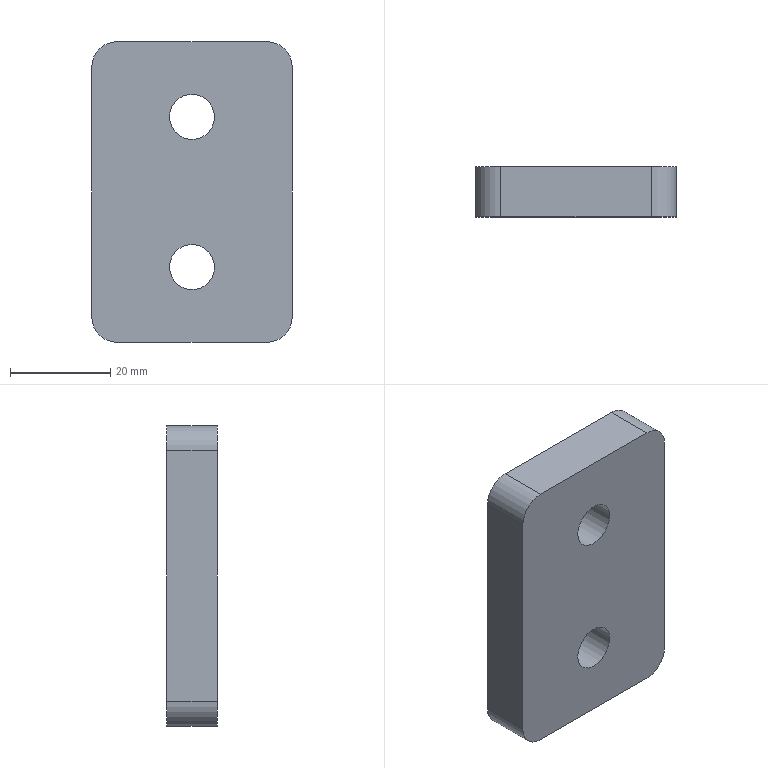Part | STEP file | SN10_002_011_PLACA | 1 solid | 12 faces | box 40 x 10 x 60 mm | volume 22513 mm3 | cylinder 6 | plane 6 | commonest cylinder face diameters 10 x4 9 x2
STEP:
#1=CARTESIAN_POINT('',(0.,0.,0.));
#2=DIRECTION('',(0.,0.,1.));
#3=DIRECTION('',(1.,0.,0.));
#4=AXIS2_PLACEMENT_3D('',#1,#2,#3);
#5=CARTESIAN_POINT('',(893.949,30.,-122.843));
#6=VERTEX_POINT('',#5);
#7=CARTESIAN_POINT('',(890.,30.,-125.));
#8=DIRECTION('',(0.,1.,0.));
#9=DIRECTION('',(1.,0.,0.));
#10=AXIS2_PLACEMENT_3D('',#7,#8,#9);
#11=CIRCLE('',#10,4.5);
#12=CARTESIAN_POINT('',(890.,29.9,-125.));
#13=DIRECTION('',(0.,-1.,0.));
#14=DIRECTION('',(0.8776,0.,0.4794));
#15=AXIS2_PLACEMENT_3D('',#12,#13,#14);
#16=CYLINDRICAL_SURFACE('',#15,4.5);
#17=CARTESIAN_POINT('',(12.066,-0.1));
#18=DIRECTION('',(-1.,0.));
#19=VECTOR('',#18,1.);
#20=LINE('',#17,#19);
#21=(GEOMETRIC_REPRESENTATION_CONTEXT(2)PARAMETRIC_REPRESENTATION_CONTEXT()REPRESENTATION_CONTEXT('',''));
#22=DEFINITIONAL_REPRESENTATION('',(#20),#21);
#23=PCURVE('',#16,#22);
#24=CARTESIAN_POINT('',(0.,30.,0.));
#25=DIRECTION('',(0.,1.,0.));
#26=DIRECTION('',(0.,0.,1.));
#27=AXIS2_PLACEMENT_3D('',#24,#25,#26);
#28=PLANE('',#27);
#29=CARTESIAN_POINT('',(-125.,890.));
#30=DIRECTION('',(0.,1.));
#31=AXIS2_PLACEMENT_2D('',#29,#30);
#32=CIRCLE('',#31,4.5);
#33=(GEOMETRIC_REPRESENTATION_CONTEXT(2)PARAMETRIC_REPRESENTATION_CONTEXT()REPRESENTATION_CONTEXT('',''));
#34=DEFINITIONAL_REPRESENTATION('',(#32),#33);
#35=PCURVE('',#28,#34);
#36=SURFACE_CURVE('',#11,(#23,#35),.PCURVE_S1.);
#37=EDGE_CURVE('',#6,#6,#36,.T.);
#38=ORIENTED_EDGE('',*,*,#37,.F.);
#39=CARTESIAN_POINT('',(893.949,20.,-122.843));
#40=VERTEX_POINT('',#39);
#41=CARTESIAN_POINT('',(893.949,30.,-122.843));
#42=CARTESIAN_POINT('',(893.949,20.,-122.843));
#43=B_SPLINE_CURVE_WITH_KNOTS('',1,(#41,#42),.UNSPECIFIED.,.F.,.F.,(2,2),(-0.1,9.9),.PIECEWISE_BEZIER_KNOTS.);
#44=CARTESIAN_POINT('',(6.283,0.));
#45=DIRECTION('',(0.,1.));
#46=VECTOR('',#45,1.);
#47=LINE('',#44,#46);
#48=(GEOMETRIC_REPRESENTATION_CONTEXT(2)PARAMETRIC_REPRESENTATION_CONTEXT()REPRESENTATION_CONTEXT('',''));
#49=DEFINITIONAL_REPRESENTATION('',(#47),#48);
#50=PCURVE('',#16,#49);
#51=CARTESIAN_POINT('',(0.,0.));
#52=DIRECTION('',(0.,1.));
#53=VECTOR('',#52,1.);
#54=LINE('',#51,#53);
#55=(GEOMETRIC_REPRESENTATION_CONTEXT(2)PARAMETRIC_REPRESENTATION_CONTEXT()REPRESENTATION_CONTEXT('',''));
#56=DEFINITIONAL_REPRESENTATION('',(#54),#55);
#57=PCURVE('',#16,#56);
#58=SEAM_CURVE('',#43,(#50,#57),.PCURVE_S1.);
#59=EDGE_CURVE('',#6,#40,#58,.T.);
#60=ORIENTED_EDGE('',*,*,#59,.T.);
#61=CARTESIAN_POINT('',(890.,20.,-125.));
#62=DIRECTION('',(0.,-1.,0.));
#63=DIRECTION('',(1.,0.,0.));
#64=AXIS2_PLACEMENT_3D('',#61,#62,#63);
#65=CIRCLE('',#64,4.5);
#66=CARTESIAN_POINT('',(-0.5,9.9));
#67=DIRECTION('',(1.,0.));
#68=VECTOR('',#67,1.);
#69=LINE('',#66,#68);
#70=(GEOMETRIC_REPRESENTATION_CONTEXT(2)PARAMETRIC_REPRESENTATION_CONTEXT()REPRESENTATION_CONTEXT('',''));
#71=DEFINITIONAL_REPRESENTATION('',(#69),#70);
#72=PCURVE('',#16,#71);
#73=CARTESIAN_POINT('',(0.,20.,0.));
#74=DIRECTION('',(0.,1.,0.));
#75=DIRECTION('',(0.,0.,1.));
#76=AXIS2_PLACEMENT_3D('',#73,#74,#75);
#77=PLANE('',#76);
#78=CARTESIAN_POINT('',(-125.,894.5));
#79=CARTESIAN_POINT('',(-117.206,894.5));
#80=CARTESIAN_POINT('',(-121.103,887.75));
#81=CARTESIAN_POINT('',(-125.,881.));
#82=CARTESIAN_POINT('',(-128.897,887.75));
#83=CARTESIAN_POINT('',(-132.794,894.5));
#84=CARTESIAN_POINT('',(-125.,894.5));
#85=(BOUNDED_CURVE()B_SPLINE_CURVE(2,(#78,#79,#80,#81,#82,#83,#84),.UNSPECIFIED.,.T.,.F.)B_SPLINE_CURVE_WITH_KNOTS((1,2,2,2,2,1),(-2.094,0.,2.094,4.189,6.283,8.378),.UNSPECIFIED.)CURVE()GEOMETRIC_REPRESENTATION_ITEM()RATIONAL_B_SPLINE_CURVE((1.,0.5,1.,0.5,1.,0.5,1.))REPRESENTATION_ITEM(''));
#86=(GEOMETRIC_REPRESENTATION_CONTEXT(2)PARAMETRIC_REPRESENTATION_CONTEXT()REPRESENTATION_CONTEXT('',''));
#87=DEFINITIONAL_REPRESENTATION('',(#85),#86);
#88=PCURVE('',#77,#87);
#89=SURFACE_CURVE('',#65,(#72,#88),.PCURVE_S1.);
#90=EDGE_CURVE('',#40,#40,#89,.T.);
#91=ORIENTED_EDGE('',*,*,#90,.F.);
#92=ORIENTED_EDGE('',*,*,#59,.F.);
#93=EDGE_LOOP('',(#38,#60,#91,#92));
#94=FACE_BOUND('',#93,.F.);
#95=ADVANCED_FACE('',(#94),#16,.F.);
#96=CARTESIAN_POINT('',(875.,30.,-140.));
#97=VERTEX_POINT('',#96);
#98=CARTESIAN_POINT('',(905.,30.,-140.));
#99=VERTEX_POINT('',#98);
#100=CARTESIAN_POINT('',(875.,30.,-140.));
#101=DIRECTION('',(1.,0.,0.));
#102=VECTOR('',#101,1.);
#103=LINE('',#100,#102);
#104=CARTESIAN_POINT('',(-140.,875.));
#105=DIRECTION('',(0.,1.));
#106=VECTOR('',#105,1.);
#107=LINE('',#104,#106);
#108=(GEOMETRIC_REPRESENTATION_CONTEXT(2)PARAMETRIC_REPRESENTATION_CONTEXT()REPRESENTATION_CONTEXT('',''));
#109=DEFINITIONAL_REPRESENTATION('',(#107),#108);
#110=PCURVE('',#28,#109);
#111=CARTESIAN_POINT('',(870.,20.,-140.));
#112=DIRECTION('',(0.,0.,1.));
#113=DIRECTION('',(1.,0.,0.));
#114=AXIS2_PLACEMENT_3D('',#111,#112,#113);
#115=PLANE('',#114);
#116=CARTESIAN_POINT('',(5.,10.));
#117=DIRECTION('',(1.,0.));
#118=VECTOR('',#117,1.);
#119=LINE('',#116,#118);
#120=(GEOMETRIC_REPRESENTATION_CONTEXT(2)PARAMETRIC_REPRESENTATION_CONTEXT()REPRESENTATION_CONTEXT('',''));
#121=DEFINITIONAL_REPRESENTATION('',(#119),#120);
#122=PCURVE('',#115,#121);
#123=SURFACE_CURVE('',#103,(#110,#122),.PCURVE_S1.);
#124=EDGE_CURVE('',#97,#99,#123,.T.);
#125=ORIENTED_EDGE('',*,*,#124,.F.);
#126=CARTESIAN_POINT('',(870.,30.,-135.));
#127=VERTEX_POINT('',#126);
#128=CARTESIAN_POINT('',(875.,30.,-135.));
#129=DIRECTION('',(0.,1.,0.));
#130=DIRECTION('',(1.,0.,0.));
#131=AXIS2_PLACEMENT_3D('',#128,#129,#130);
#132=CIRCLE('',#131,5.);
#133=CARTESIAN_POINT('',(-135.,875.));
#134=DIRECTION('',(0.,1.));
#135=AXIS2_PLACEMENT_2D('',#133,#134);
#136=CIRCLE('',#135,5.);
#137=(GEOMETRIC_REPRESENTATION_CONTEXT(2)PARAMETRIC_REPRESENTATION_CONTEXT()REPRESENTATION_CONTEXT('',''));
#138=DEFINITIONAL_REPRESENTATION('',(#136),#137);
#139=PCURVE('',#28,#138);
#140=CARTESIAN_POINT('',(875.,25.,-135.));
#141=DIRECTION('',(0.,1.,0.));
#142=DIRECTION('',(0.,0.,-1.));
#143=AXIS2_PLACEMENT_3D('',#140,#141,#142);
#144=CYLINDRICAL_SURFACE('',#143,5.);
#145=CARTESIAN_POINT('',(-1.571,5.));
#146=DIRECTION('',(1.,0.));
#147=VECTOR('',#146,1.);
#148=LINE('',#145,#147);
#149=(GEOMETRIC_REPRESENTATION_CONTEXT(2)PARAMETRIC_REPRESENTATION_CONTEXT()REPRESENTATION_CONTEXT('',''));
#150=DEFINITIONAL_REPRESENTATION('',(#148),#149);
#151=PCURVE('',#144,#150);
#152=SURFACE_CURVE('',#132,(#139,#151),.PCURVE_S1.);
#153=EDGE_CURVE('',#97,#127,#152,.T.);
#154=ORIENTED_EDGE('',*,*,#153,.T.);
#155=CARTESIAN_POINT('',(870.,30.,-85.));
#156=VERTEX_POINT('',#155);
#157=CARTESIAN_POINT('',(870.,30.,-85.));
#158=DIRECTION('',(0.,0.,-1.));
#159=VECTOR('',#158,1.);
#160=LINE('',#157,#159);
#161=CARTESIAN_POINT('',(-85.,870.));
#162=DIRECTION('',(-1.,0.));
#163=VECTOR('',#162,1.);
#164=LINE('',#161,#163);
#165=(GEOMETRIC_REPRESENTATION_CONTEXT(2)PARAMETRIC_REPRESENTATION_CONTEXT()REPRESENTATION_CONTEXT('',''));
#166=DEFINITIONAL_REPRESENTATION('',(#164),#165);
#167=PCURVE('',#28,#166);
#168=CARTESIAN_POINT('',(870.,20.,-80.));
#169=DIRECTION('',(1.,0.,0.));
#170=DIRECTION('',(0.,0.,-1.));
#171=AXIS2_PLACEMENT_3D('',#168,#169,#170);
#172=PLANE('',#171);
#173=CARTESIAN_POINT('',(5.,10.));
#174=DIRECTION('',(1.,0.));
#175=VECTOR('',#174,1.);
#176=LINE('',#173,#175);
#177=(GEOMETRIC_REPRESENTATION_CONTEXT(2)PARAMETRIC_REPRESENTATION_CONTEXT()REPRESENTATION_CONTEXT('',''));
#178=DEFINITIONAL_REPRESENTATION('',(#176),#177);
#179=PCURVE('',#172,#178);
#180=SURFACE_CURVE('',#160,(#167,#179),.PCURVE_S1.);
#181=EDGE_CURVE('',#156,#127,#180,.T.);
#182=ORIENTED_EDGE('',*,*,#181,.F.);
#183=CARTESIAN_POINT('',(875.,30.,-80.));
#184=VERTEX_POINT('',#183);
#185=CARTESIAN_POINT('',(875.,30.,-85.));
#186=DIRECTION('',(0.,1.,0.));
#187=DIRECTION('',(1.,0.,0.));
#188=AXIS2_PLACEMENT_3D('',#185,#186,#187);
#189=CIRCLE('',#188,5.);
#190=CARTESIAN_POINT('',(-85.,875.));
#191=DIRECTION('',(0.,1.));
#192=AXIS2_PLACEMENT_2D('',#190,#191);
#193=CIRCLE('',#192,5.);
#194=(GEOMETRIC_REPRESENTATION_CONTEXT(2)PARAMETRIC_REPRESENTATION_CONTEXT()REPRESENTATION_CONTEXT('',''));
#195=DEFINITIONAL_REPRESENTATION('',(#193),#194);
#196=PCURVE('',#28,#195);
#197=CARTESIAN_POINT('',(875.,25.,-85.));
#198=DIRECTION('',(0.,1.,0.));
#199=DIRECTION('',(-1.,0.,0.));
#200=AXIS2_PLACEMENT_3D('',#197,#198,#199);
#201=CYLINDRICAL_SURFACE('',#200,5.);
#202=CARTESIAN_POINT('',(-3.142,5.));
#203=DIRECTION('',(1.,0.));
#204=VECTOR('',#203,1.);
#205=LINE('',#202,#204);
#206=(GEOMETRIC_REPRESENTATION_CONTEXT(2)PARAMETRIC_REPRESENTATION_CONTEXT()REPRESENTATION_CONTEXT('',''));
#207=DEFINITIONAL_REPRESENTATION('',(#205),#206);
#208=PCURVE('',#201,#207);
#209=SURFACE_CURVE('',#189,(#196,#208),.PCURVE_S1.);
#210=EDGE_CURVE('',#156,#184,#209,.T.);
#211=ORIENTED_EDGE('',*,*,#210,.T.);
#212=CARTESIAN_POINT('',(905.,30.,-80.));
#213=VERTEX_POINT('',#212);
#214=CARTESIAN_POINT('',(905.,30.,-80.));
#215=DIRECTION('',(-1.,0.,0.));
#216=VECTOR('',#215,1.);
#217=LINE('',#214,#216);
#218=CARTESIAN_POINT('',(-80.,905.));
#219=DIRECTION('',(0.,-1.));
#220=VECTOR('',#219,1.);
#221=LINE('',#218,#220);
#222=(GEOMETRIC_REPRESENTATION_CONTEXT(2)PARAMETRIC_REPRESENTATION_CONTEXT()REPRESENTATION_CONTEXT('',''));
#223=DEFINITIONAL_REPRESENTATION('',(#221),#222);
#224=PCURVE('',#28,#223);
#225=CARTESIAN_POINT('',(910.,20.,-80.));
#226=DIRECTION('',(0.,0.,-1.));
#227=DIRECTION('',(-1.,0.,0.));
#228=AXIS2_PLACEMENT_3D('',#225,#226,#227);
#229=PLANE('',#228);
#230=CARTESIAN_POINT('',(5.,10.));
#231=DIRECTION('',(1.,0.));
#232=VECTOR('',#231,1.);
#233=LINE('',#230,#232);
#234=(GEOMETRIC_REPRESENTATION_CONTEXT(2)PARAMETRIC_REPRESENTATION_CONTEXT()REPRESENTATION_CONTEXT('',''));
#235=DEFINITIONAL_REPRESENTATION('',(#233),#234);
#236=PCURVE('',#229,#235);
#237=SURFACE_CURVE('',#217,(#224,#236),.PCURVE_S1.);
#238=EDGE_CURVE('',#213,#184,#237,.T.);
#239=ORIENTED_EDGE('',*,*,#238,.F.);
#240=CARTESIAN_POINT('',(910.,30.,-85.));
#241=VERTEX_POINT('',#240);
#242=CARTESIAN_POINT('',(905.,30.,-85.));
#243=DIRECTION('',(0.,1.,0.));
#244=DIRECTION('',(1.,0.,0.));
#245=AXIS2_PLACEMENT_3D('',#242,#243,#244);
#246=CIRCLE('',#245,5.);
#247=CARTESIAN_POINT('',(-85.,905.));
#248=DIRECTION('',(0.,1.));
#249=AXIS2_PLACEMENT_2D('',#247,#248);
#250=CIRCLE('',#249,5.);
#251=(GEOMETRIC_REPRESENTATION_CONTEXT(2)PARAMETRIC_REPRESENTATION_CONTEXT()REPRESENTATION_CONTEXT('',''));
#252=DEFINITIONAL_REPRESENTATION('',(#250),#251);
#253=PCURVE('',#28,#252);
#254=CARTESIAN_POINT('',(905.,25.,-85.));
#255=DIRECTION('',(0.,1.,0.));
#256=DIRECTION('',(0.,0.,1.));
#257=AXIS2_PLACEMENT_3D('',#254,#255,#256);
#258=CYLINDRICAL_SURFACE('',#257,5.);
#259=CARTESIAN_POINT('',(-4.712,5.));
#260=DIRECTION('',(1.,0.));
#261=VECTOR('',#260,1.);
#262=LINE('',#259,#261);
#263=(GEOMETRIC_REPRESENTATION_CONTEXT(2)PARAMETRIC_REPRESENTATION_CONTEXT()REPRESENTATION_CONTEXT('',''));
#264=DEFINITIONAL_REPRESENTATION('',(#262),#263);
#265=PCURVE('',#258,#264);
#266=SURFACE_CURVE('',#246,(#253,#265),.PCURVE_S1.);
#267=EDGE_CURVE('',#213,#241,#266,.T.);
#268=ORIENTED_EDGE('',*,*,#267,.T.);
#269=CARTESIAN_POINT('',(910.,30.,-135.));
#270=VERTEX_POINT('',#269);
#271=CARTESIAN_POINT('',(910.,30.,-135.));
#272=DIRECTION('',(0.,0.,1.));
#273=VECTOR('',#272,1.);
#274=LINE('',#271,#273);
#275=CARTESIAN_POINT('',(-135.,910.));
#276=DIRECTION('',(1.,0.));
#277=VECTOR('',#276,1.);
#278=LINE('',#275,#277);
#279=(GEOMETRIC_REPRESENTATION_CONTEXT(2)PARAMETRIC_REPRESENTATION_CONTEXT()REPRESENTATION_CONTEXT('',''));
#280=DEFINITIONAL_REPRESENTATION('',(#278),#279);
#281=PCURVE('',#28,#280);
#282=CARTESIAN_POINT('',(910.,20.,-140.));
#283=DIRECTION('',(-1.,0.,0.));
#284=DIRECTION('',(0.,0.,1.));
#285=AXIS2_PLACEMENT_3D('',#282,#283,#284);
#286=PLANE('',#285);
#287=CARTESIAN_POINT('',(5.,10.));
#288=DIRECTION('',(1.,0.));
#289=VECTOR('',#288,1.);
#290=LINE('',#287,#289);
#291=(GEOMETRIC_REPRESENTATION_CONTEXT(2)PARAMETRIC_REPRESENTATION_CONTEXT()REPRESENTATION_CONTEXT('',''));
#292=DEFINITIONAL_REPRESENTATION('',(#290),#291);
#293=PCURVE('',#286,#292);
#294=SURFACE_CURVE('',#274,(#281,#293),.PCURVE_S1.);
#295=EDGE_CURVE('',#270,#241,#294,.T.);
#296=ORIENTED_EDGE('',*,*,#295,.F.);
#297=CARTESIAN_POINT('',(905.,30.,-135.));
#298=DIRECTION('',(0.,1.,0.));
#299=DIRECTION('',(1.,0.,0.));
#300=AXIS2_PLACEMENT_3D('',#297,#298,#299);
#301=CIRCLE('',#300,5.);
#302=CARTESIAN_POINT('',(-135.,905.));
#303=DIRECTION('',(0.,1.));
#304=AXIS2_PLACEMENT_2D('',#302,#303);
#305=CIRCLE('',#304,5.);
#306=(GEOMETRIC_REPRESENTATION_CONTEXT(2)PARAMETRIC_REPRESENTATION_CONTEXT()REPRESENTATION_CONTEXT('',''));
#307=DEFINITIONAL_REPRESENTATION('',(#305),#306);
#308=PCURVE('',#28,#307);
#309=CARTESIAN_POINT('',(905.,25.,-135.));
#310=DIRECTION('',(0.,1.,0.));
#311=DIRECTION('',(1.,0.,0.));
#312=AXIS2_PLACEMENT_3D('',#309,#310,#311);
#313=CYLINDRICAL_SURFACE('',#312,5.);
#314=CARTESIAN_POINT('',(0.,5.));
#315=DIRECTION('',(1.,0.));
#316=VECTOR('',#315,1.);
#317=LINE('',#314,#316);
#318=(GEOMETRIC_REPRESENTATION_CONTEXT(2)PARAMETRIC_REPRESENTATION_CONTEXT()REPRESENTATION_CONTEXT('',''));
#319=DEFINITIONAL_REPRESENTATION('',(#317),#318);
#320=PCURVE('',#313,#319);
#321=SURFACE_CURVE('',#301,(#308,#320),.PCURVE_S1.);
#322=EDGE_CURVE('',#270,#99,#321,.T.);
#323=ORIENTED_EDGE('',*,*,#322,.T.);
#324=EDGE_LOOP('',(#125,#154,#182,#211,#239,#268,#296,#323));
#325=FACE_BOUND('',#324,.T.);
#326=ORIENTED_EDGE('',*,*,#37,.F.);
#327=EDGE_LOOP('',(#326));
#328=FACE_BOUND('',#327,.T.);
#329=CARTESIAN_POINT('',(893.949,30.,-92.843));
#330=VERTEX_POINT('',#329);
#331=CARTESIAN_POINT('',(890.,30.,-95.));
#332=DIRECTION('',(0.,1.,0.));
#333=DIRECTION('',(1.,0.,0.));
#334=AXIS2_PLACEMENT_3D('',#331,#332,#333);
#335=CIRCLE('',#334,4.5);
#336=CARTESIAN_POINT('',(-95.,890.));
#337=DIRECTION('',(0.,1.));
#338=AXIS2_PLACEMENT_2D('',#336,#337);
#339=CIRCLE('',#338,4.5);
#340=(GEOMETRIC_REPRESENTATION_CONTEXT(2)PARAMETRIC_REPRESENTATION_CONTEXT()REPRESENTATION_CONTEXT('',''));
#341=DEFINITIONAL_REPRESENTATION('',(#339),#340);
#342=PCURVE('',#28,#341);
#343=CARTESIAN_POINT('',(890.,29.9,-95.));
#344=DIRECTION('',(0.,-1.,0.));
#345=DIRECTION('',(0.8776,0.,0.4794));
#346=AXIS2_PLACEMENT_3D('',#343,#344,#345);
#347=CYLINDRICAL_SURFACE('',#346,4.5);
#348=CARTESIAN_POINT('',(12.066,-0.1));
#349=DIRECTION('',(-1.,0.));
#350=VECTOR('',#349,1.);
#351=LINE('',#348,#350);
#352=(GEOMETRIC_REPRESENTATION_CONTEXT(2)PARAMETRIC_REPRESENTATION_CONTEXT()REPRESENTATION_CONTEXT('',''));
#353=DEFINITIONAL_REPRESENTATION('',(#351),#352);
#354=PCURVE('',#347,#353);
#355=SURFACE_CURVE('',#335,(#342,#354),.PCURVE_S1.);
#356=EDGE_CURVE('',#330,#330,#355,.T.);
#357=ORIENTED_EDGE('',*,*,#356,.F.);
#358=EDGE_LOOP('',(#357));
#359=FACE_BOUND('',#358,.T.);
#360=ADVANCED_FACE('',(#325,#328,#359),#28,.T.);
#361=CARTESIAN_POINT('',(905.,20.,-140.));
#362=VERTEX_POINT('',#361);
#363=CARTESIAN_POINT('',(905.,20.,-140.));
#364=DIRECTION('',(0.,1.,0.));
#365=VECTOR('',#364,1.);
#366=LINE('',#363,#365);
#367=CARTESIAN_POINT('',(35.,0.));
#368=DIRECTION('',(0.,1.));
#369=VECTOR('',#368,1.);
#370=LINE('',#367,#369);
#371=(GEOMETRIC_REPRESENTATION_CONTEXT(2)PARAMETRIC_REPRESENTATION_CONTEXT()REPRESENTATION_CONTEXT('',''));
#372=DEFINITIONAL_REPRESENTATION('',(#370),#371);
#373=PCURVE('',#115,#372);
#374=CARTESIAN_POINT('',(1.571,-5.));
#375=DIRECTION('',(0.,1.));
#376=VECTOR('',#375,1.);
#377=LINE('',#374,#376);
#378=(GEOMETRIC_REPRESENTATION_CONTEXT(2)PARAMETRIC_REPRESENTATION_CONTEXT()REPRESENTATION_CONTEXT('',''));
#379=DEFINITIONAL_REPRESENTATION('',(#377),#378);
#380=PCURVE('',#313,#379);
#381=SURFACE_CURVE('',#366,(#373,#380),.PCURVE_S1.);
#382=EDGE_CURVE('',#362,#99,#381,.T.);
#383=ORIENTED_EDGE('',*,*,#382,.F.);
#384=CARTESIAN_POINT('',(875.,20.,-140.));
#385=VERTEX_POINT('',#384);
#386=CARTESIAN_POINT('',(875.,20.,-140.));
#387=DIRECTION('',(1.,0.,0.));
#388=VECTOR('',#387,1.);
#389=LINE('',#386,#388);
#390=CARTESIAN_POINT('',(5.,0.));
#391=DIRECTION('',(1.,0.));
#392=VECTOR('',#391,1.);
#393=LINE('',#390,#392);
#394=(GEOMETRIC_REPRESENTATION_CONTEXT(2)PARAMETRIC_REPRESENTATION_CONTEXT()REPRESENTATION_CONTEXT('',''));
#395=DEFINITIONAL_REPRESENTATION('',(#393),#394);
#396=PCURVE('',#115,#395);
#397=CARTESIAN_POINT('',(-140.,875.));
#398=DIRECTION('',(0.,1.));
#399=VECTOR('',#398,1.);
#400=LINE('',#397,#399);
#401=(GEOMETRIC_REPRESENTATION_CONTEXT(2)PARAMETRIC_REPRESENTATION_CONTEXT()REPRESENTATION_CONTEXT('',''));
#402=DEFINITIONAL_REPRESENTATION('',(#400),#401);
#403=PCURVE('',#77,#402);
#404=SURFACE_CURVE('',#389,(#396,#403),.PCURVE_S1.);
#405=EDGE_CURVE('',#385,#362,#404,.T.);
#406=ORIENTED_EDGE('',*,*,#405,.F.);
#407=CARTESIAN_POINT('',(875.,20.,-140.));
#408=DIRECTION('',(0.,1.,0.));
#409=VECTOR('',#408,1.);
#410=LINE('',#407,#409);
#411=CARTESIAN_POINT('',(5.,0.));
#412=DIRECTION('',(0.,1.));
#413=VECTOR('',#412,1.);
#414=LINE('',#411,#413);
#415=(GEOMETRIC_REPRESENTATION_CONTEXT(2)PARAMETRIC_REPRESENTATION_CONTEXT()REPRESENTATION_CONTEXT('',''));
#416=DEFINITIONAL_REPRESENTATION('',(#414),#415);
#417=PCURVE('',#115,#416);
#418=CARTESIAN_POINT('',(0.,-5.));
#419=DIRECTION('',(0.,1.));
#420=VECTOR('',#419,1.);
#421=LINE('',#418,#420);
#422=(GEOMETRIC_REPRESENTATION_CONTEXT(2)PARAMETRIC_REPRESENTATION_CONTEXT()REPRESENTATION_CONTEXT('',''));
#423=DEFINITIONAL_REPRESENTATION('',(#421),#422);
#424=PCURVE('',#144,#423);
#425=SURFACE_CURVE('',#410,(#417,#424),.PCURVE_S1.);
#426=EDGE_CURVE('',#385,#97,#425,.T.);
#427=ORIENTED_EDGE('',*,*,#426,.T.);
#428=ORIENTED_EDGE('',*,*,#124,.T.);
#429=EDGE_LOOP('',(#383,#406,#427,#428));
#430=FACE_BOUND('',#429,.T.);
#431=ADVANCED_FACE('',(#430),#115,.F.);
#432=CARTESIAN_POINT('',(870.,20.,-135.));
#433=VERTEX_POINT('',#432);
#434=CARTESIAN_POINT('',(870.,20.,-135.));
#435=DIRECTION('',(0.,1.,0.));
#436=VECTOR('',#435,1.);
#437=LINE('',#434,#436);
#438=CARTESIAN_POINT('',(55.,0.));
#439=DIRECTION('',(0.,1.));
#440=VECTOR('',#439,1.);
#441=LINE('',#438,#440);
#442=(GEOMETRIC_REPRESENTATION_CONTEXT(2)PARAMETRIC_REPRESENTATION_CONTEXT()REPRESENTATION_CONTEXT('',''));
#443=DEFINITIONAL_REPRESENTATION('',(#441),#442);
#444=PCURVE('',#172,#443);
#445=CARTESIAN_POINT('',(1.571,-5.));
#446=DIRECTION('',(0.,1.));
#447=VECTOR('',#446,1.);
#448=LINE('',#445,#447);
#449=(GEOMETRIC_REPRESENTATION_CONTEXT(2)PARAMETRIC_REPRESENTATION_CONTEXT()REPRESENTATION_CONTEXT('',''));
#450=DEFINITIONAL_REPRESENTATION('',(#448),#449);
#451=PCURVE('',#144,#450);
#452=SURFACE_CURVE('',#437,(#444,#451),.PCURVE_S1.);
#453=EDGE_CURVE('',#433,#127,#452,.T.);
#454=ORIENTED_EDGE('',*,*,#453,.F.);
#455=CARTESIAN_POINT('',(870.,20.,-85.));
#456=VERTEX_POINT('',#455);
#457=CARTESIAN_POINT('',(870.,20.,-85.));
#458=DIRECTION('',(0.,0.,-1.));
#459=VECTOR('',#458,1.);
#460=LINE('',#457,#459);
#461=CARTESIAN_POINT('',(5.,0.));
#462=DIRECTION('',(1.,0.));
#463=VECTOR('',#462,1.);
#464=LINE('',#461,#463);
#465=(GEOMETRIC_REPRESENTATION_CONTEXT(2)PARAMETRIC_REPRESENTATION_CONTEXT()REPRESENTATION_CONTEXT('',''));
#466=DEFINITIONAL_REPRESENTATION('',(#464),#465);
#467=PCURVE('',#172,#466);
#468=CARTESIAN_POINT('',(-85.,870.));
#469=DIRECTION('',(-1.,0.));
#470=VECTOR('',#469,1.);
#471=LINE('',#468,#470);
#472=(GEOMETRIC_REPRESENTATION_CONTEXT(2)PARAMETRIC_REPRESENTATION_CONTEXT()REPRESENTATION_CONTEXT('',''));
#473=DEFINITIONAL_REPRESENTATION('',(#471),#472);
#474=PCURVE('',#77,#473);
#475=SURFACE_CURVE('',#460,(#467,#474),.PCURVE_S1.);
#476=EDGE_CURVE('',#456,#433,#475,.T.);
#477=ORIENTED_EDGE('',*,*,#476,.F.);
#478=CARTESIAN_POINT('',(870.,20.,-85.));
#479=DIRECTION('',(0.,1.,0.));
#480=VECTOR('',#479,1.);
#481=LINE('',#478,#480);
#482=CARTESIAN_POINT('',(5.,0.));
#483=DIRECTION('',(0.,1.));
#484=VECTOR('',#483,1.);
#485=LINE('',#482,#484);
#486=(GEOMETRIC_REPRESENTATION_CONTEXT(2)PARAMETRIC_REPRESENTATION_CONTEXT()REPRESENTATION_CONTEXT('',''));
#487=DEFINITIONAL_REPRESENTATION('',(#485),#486);
#488=PCURVE('',#172,#487);
#489=CARTESIAN_POINT('',(0.,-5.));
#490=DIRECTION('',(0.,1.));
#491=VECTOR('',#490,1.);
#492=LINE('',#489,#491);
#493=(GEOMETRIC_REPRESENTATION_CONTEXT(2)PARAMETRIC_REPRESENTATION_CONTEXT()REPRESENTATION_CONTEXT('',''));
#494=DEFINITIONAL_REPRESENTATION('',(#492),#493);
#495=PCURVE('',#201,#494);
#496=SURFACE_CURVE('',#481,(#488,#495),.PCURVE_S1.);
#497=EDGE_CURVE('',#456,#156,#496,.T.);
#498=ORIENTED_EDGE('',*,*,#497,.T.);
#499=ORIENTED_EDGE('',*,*,#181,.T.);
#500=EDGE_LOOP('',(#454,#477,#498,#499));
#501=FACE_BOUND('',#500,.T.);
#502=ADVANCED_FACE('',(#501),#172,.F.);
#503=CARTESIAN_POINT('',(875.,20.,-80.));
#504=VERTEX_POINT('',#503);
#505=CARTESIAN_POINT('',(875.,20.,-80.));
#506=DIRECTION('',(0.,1.,0.));
#507=VECTOR('',#506,1.);
#508=LINE('',#505,#507);
#509=CARTESIAN_POINT('',(35.,0.));
#510=DIRECTION('',(0.,1.));
#511=VECTOR('',#510,1.);
#512=LINE('',#509,#511);
#513=(GEOMETRIC_REPRESENTATION_CONTEXT(2)PARAMETRIC_REPRESENTATION_CONTEXT()REPRESENTATION_CONTEXT('',''));
#514=DEFINITIONAL_REPRESENTATION('',(#512),#513);
#515=PCURVE('',#229,#514);
#516=CARTESIAN_POINT('',(1.571,-5.));
#517=DIRECTION('',(0.,1.));
#518=VECTOR('',#517,1.);
#519=LINE('',#516,#518);
#520=(GEOMETRIC_REPRESENTATION_CONTEXT(2)PARAMETRIC_REPRESENTATION_CONTEXT()REPRESENTATION_CONTEXT('',''));
#521=DEFINITIONAL_REPRESENTATION('',(#519),#520);
#522=PCURVE('',#201,#521);
#523=SURFACE_CURVE('',#508,(#515,#522),.PCURVE_S1.);
#524=EDGE_CURVE('',#504,#184,#523,.T.);
#525=ORIENTED_EDGE('',*,*,#524,.F.);
#526=CARTESIAN_POINT('',(905.,20.,-80.));
#527=VERTEX_POINT('',#526);
#528=CARTESIAN_POINT('',(905.,20.,-80.));
#529=DIRECTION('',(-1.,0.,0.));
#530=VECTOR('',#529,1.);
#531=LINE('',#528,#530);
#532=CARTESIAN_POINT('',(5.,0.));
#533=DIRECTION('',(1.,0.));
#534=VECTOR('',#533,1.);
#535=LINE('',#532,#534);
#536=(GEOMETRIC_REPRESENTATION_CONTEXT(2)PARAMETRIC_REPRESENTATION_CONTEXT()REPRESENTATION_CONTEXT('',''));
#537=DEFINITIONAL_REPRESENTATION('',(#535),#536);
#538=PCURVE('',#229,#537);
#539=CARTESIAN_POINT('',(-80.,905.));
#540=DIRECTION('',(0.,-1.));
#541=VECTOR('',#540,1.);
#542=LINE('',#539,#541);
#543=(GEOMETRIC_REPRESENTATION_CONTEXT(2)PARAMETRIC_REPRESENTATION_CONTEXT()REPRESENTATION_CONTEXT('',''));
#544=DEFINITIONAL_REPRESENTATION('',(#542),#543);
#545=PCURVE('',#77,#544);
#546=SURFACE_CURVE('',#531,(#538,#545),.PCURVE_S1.);
#547=EDGE_CURVE('',#527,#504,#546,.T.);
#548=ORIENTED_EDGE('',*,*,#547,.F.);
#549=CARTESIAN_POINT('',(905.,20.,-80.));
#550=DIRECTION('',(0.,1.,0.));
#551=VECTOR('',#550,1.);
#552=LINE('',#549,#551);
#553=CARTESIAN_POINT('',(5.,0.));
#554=DIRECTION('',(0.,1.));
#555=VECTOR('',#554,1.);
#556=LINE('',#553,#555);
#557=(GEOMETRIC_REPRESENTATION_CONTEXT(2)PARAMETRIC_REPRESENTATION_CONTEXT()REPRESENTATION_CONTEXT('',''));
#558=DEFINITIONAL_REPRESENTATION('',(#556),#557);
#559=PCURVE('',#229,#558);
#560=CARTESIAN_POINT('',(0.,-5.));
#561=DIRECTION('',(0.,1.));
#562=VECTOR('',#561,1.);
#563=LINE('',#560,#562);
#564=(GEOMETRIC_REPRESENTATION_CONTEXT(2)PARAMETRIC_REPRESENTATION_CONTEXT()REPRESENTATION_CONTEXT('',''));
#565=DEFINITIONAL_REPRESENTATION('',(#563),#564);
#566=PCURVE('',#258,#565);
#567=SURFACE_CURVE('',#552,(#559,#566),.PCURVE_S1.);
#568=EDGE_CURVE('',#527,#213,#567,.T.);
#569=ORIENTED_EDGE('',*,*,#568,.T.);
#570=ORIENTED_EDGE('',*,*,#238,.T.);
#571=EDGE_LOOP('',(#525,#548,#569,#570));
#572=FACE_BOUND('',#571,.T.);
#573=ADVANCED_FACE('',(#572),#229,.F.);
#574=CARTESIAN_POINT('',(910.,20.,-135.));
#575=VERTEX_POINT('',#574);
#576=CARTESIAN_POINT('',(910.,20.,-135.));
#577=DIRECTION('',(0.,1.,0.));
#578=VECTOR('',#577,1.);
#579=LINE('',#576,#578);
#580=CARTESIAN_POINT('',(5.,0.));
#581=DIRECTION('',(0.,1.));
#582=VECTOR('',#581,1.);
#583=LINE('',#580,#582);
#584=(GEOMETRIC_REPRESENTATION_CONTEXT(2)PARAMETRIC_REPRESENTATION_CONTEXT()REPRESENTATION_CONTEXT('',''));
#585=DEFINITIONAL_REPRESENTATION('',(#583),#584);
#586=PCURVE('',#286,#585);
#587=CARTESIAN_POINT('',(0.,-5.));
#588=DIRECTION('',(0.,1.));
#589=VECTOR('',#588,1.);
#590=LINE('',#587,#589);
#591=(GEOMETRIC_REPRESENTATION_CONTEXT(2)PARAMETRIC_REPRESENTATION_CONTEXT()REPRESENTATION_CONTEXT('',''));
#592=DEFINITIONAL_REPRESENTATION('',(#590),#591);
#593=PCURVE('',#313,#592);
#594=SURFACE_CURVE('',#579,(#586,#593),.PCURVE_S1.);
#595=EDGE_CURVE('',#575,#270,#594,.T.);
#596=ORIENTED_EDGE('',*,*,#595,.T.);
#597=ORIENTED_EDGE('',*,*,#295,.T.);
#598=CARTESIAN_POINT('',(910.,20.,-85.));
#599=VERTEX_POINT('',#598);
#600=CARTESIAN_POINT('',(910.,20.,-85.));
#601=DIRECTION('',(0.,1.,0.));
#602=VECTOR('',#601,1.);
#603=LINE('',#600,#602);
#604=CARTESIAN_POINT('',(55.,0.));
#605=DIRECTION('',(0.,1.));
#606=VECTOR('',#605,1.);
#607=LINE('',#604,#606);
#608=(GEOMETRIC_REPRESENTATION_CONTEXT(2)PARAMETRIC_REPRESENTATION_CONTEXT()REPRESENTATION_CONTEXT('',''));
#609=DEFINITIONAL_REPRESENTATION('',(#607),#608);
#610=PCURVE('',#286,#609);
#611=CARTESIAN_POINT('',(1.571,-5.));
#612=DIRECTION('',(0.,1.));
#613=VECTOR('',#612,1.);
#614=LINE('',#611,#613);
#615=(GEOMETRIC_REPRESENTATION_CONTEXT(2)PARAMETRIC_REPRESENTATION_CONTEXT()REPRESENTATION_CONTEXT('',''));
#616=DEFINITIONAL_REPRESENTATION('',(#614),#615);
#617=PCURVE('',#258,#616);
#618=SURFACE_CURVE('',#603,(#610,#617),.PCURVE_S1.);
#619=EDGE_CURVE('',#599,#241,#618,.T.);
#620=ORIENTED_EDGE('',*,*,#619,.F.);
#621=CARTESIAN_POINT('',(910.,20.,-135.));
#622=DIRECTION('',(0.,0.,1.));
#623=VECTOR('',#622,1.);
#624=LINE('',#621,#623);
#625=CARTESIAN_POINT('',(5.,0.));
#626=DIRECTION('',(1.,0.));
#627=VECTOR('',#626,1.);
#628=LINE('',#625,#627);
#629=(GEOMETRIC_REPRESENTATION_CONTEXT(2)PARAMETRIC_REPRESENTATION_CONTEXT()REPRESENTATION_CONTEXT('',''));
#630=DEFINITIONAL_REPRESENTATION('',(#628),#629);
#631=PCURVE('',#286,#630);
#632=CARTESIAN_POINT('',(-135.,910.));
#633=DIRECTION('',(1.,0.));
#634=VECTOR('',#633,1.);
#635=LINE('',#632,#634);
#636=(GEOMETRIC_REPRESENTATION_CONTEXT(2)PARAMETRIC_REPRESENTATION_CONTEXT()REPRESENTATION_CONTEXT('',''));
#637=DEFINITIONAL_REPRESENTATION('',(#635),#636);
#638=PCURVE('',#77,#637);
#639=SURFACE_CURVE('',#624,(#631,#638),.PCURVE_S1.);
#640=EDGE_CURVE('',#575,#599,#639,.T.);
#641=ORIENTED_EDGE('',*,*,#640,.F.);
#642=EDGE_LOOP('',(#596,#597,#620,#641));
#643=FACE_BOUND('',#642,.T.);
#644=ADVANCED_FACE('',(#643),#286,.F.);
#645=ORIENTED_EDGE('',*,*,#356,.F.);
#646=CARTESIAN_POINT('',(893.949,20.,-92.843));
#647=VERTEX_POINT('',#646);
#648=CARTESIAN_POINT('',(893.949,30.,-92.843));
#649=CARTESIAN_POINT('',(893.949,20.,-92.843));
#650=B_SPLINE_CURVE_WITH_KNOTS('',1,(#648,#649),.UNSPECIFIED.,.F.,.F.,(2,2),(-0.1,9.9),.PIECEWISE_BEZIER_KNOTS.);
#651=CARTESIAN_POINT('',(6.283,0.));
#652=DIRECTION('',(0.,1.));
#653=VECTOR('',#652,1.);
#654=LINE('',#651,#653);
#655=(GEOMETRIC_REPRESENTATION_CONTEXT(2)PARAMETRIC_REPRESENTATION_CONTEXT()REPRESENTATION_CONTEXT('',''));
#656=DEFINITIONAL_REPRESENTATION('',(#654),#655);
#657=PCURVE('',#347,#656);
#658=CARTESIAN_POINT('',(0.,0.));
#659=DIRECTION('',(0.,1.));
#660=VECTOR('',#659,1.);
#661=LINE('',#658,#660);
#662=(GEOMETRIC_REPRESENTATION_CONTEXT(2)PARAMETRIC_REPRESENTATION_CONTEXT()REPRESENTATION_CONTEXT('',''));
#663=DEFINITIONAL_REPRESENTATION('',(#661),#662);
#664=PCURVE('',#347,#663);
#665=SEAM_CURVE('',#650,(#657,#664),.PCURVE_S1.);
#666=EDGE_CURVE('',#330,#647,#665,.T.);
#667=ORIENTED_EDGE('',*,*,#666,.T.);
#668=CARTESIAN_POINT('',(890.,20.,-95.));
#669=DIRECTION('',(0.,-1.,0.));
#670=DIRECTION('',(1.,0.,0.));
#671=AXIS2_PLACEMENT_3D('',#668,#669,#670);
#672=CIRCLE('',#671,4.5);
#673=CARTESIAN_POINT('',(-0.5,9.9));
#674=DIRECTION('',(1.,0.));
#675=VECTOR('',#674,1.);
#676=LINE('',#673,#675);
#677=(GEOMETRIC_REPRESENTATION_CONTEXT(2)PARAMETRIC_REPRESENTATION_CONTEXT()REPRESENTATION_CONTEXT('',''));
#678=DEFINITIONAL_REPRESENTATION('',(#676),#677);
#679=PCURVE('',#347,#678);
#680=CARTESIAN_POINT('',(-95.,894.5));
#681=CARTESIAN_POINT('',(-87.206,894.5));
#682=CARTESIAN_POINT('',(-91.103,887.75));
#683=CARTESIAN_POINT('',(-95.,881.));
#684=CARTESIAN_POINT('',(-98.897,887.75));
#685=CARTESIAN_POINT('',(-102.794,894.5));
#686=CARTESIAN_POINT('',(-95.,894.5));
#687=(BOUNDED_CURVE()B_SPLINE_CURVE(2,(#680,#681,#682,#683,#684,#685,#686),.UNSPECIFIED.,.T.,.F.)B_SPLINE_CURVE_WITH_KNOTS((1,2,2,2,2,1),(-2.094,0.,2.094,4.189,6.283,8.378),.UNSPECIFIED.)CURVE()GEOMETRIC_REPRESENTATION_ITEM()RATIONAL_B_SPLINE_CURVE((1.,0.5,1.,0.5,1.,0.5,1.))REPRESENTATION_ITEM(''));
#688=(GEOMETRIC_REPRESENTATION_CONTEXT(2)PARAMETRIC_REPRESENTATION_CONTEXT()REPRESENTATION_CONTEXT('',''));
#689=DEFINITIONAL_REPRESENTATION('',(#687),#688);
#690=PCURVE('',#77,#689);
#691=SURFACE_CURVE('',#672,(#679,#690),.PCURVE_S1.);
#692=EDGE_CURVE('',#647,#647,#691,.T.);
#693=ORIENTED_EDGE('',*,*,#692,.F.);
#694=ORIENTED_EDGE('',*,*,#666,.F.);
#695=EDGE_LOOP('',(#645,#667,#693,#694));
#696=FACE_BOUND('',#695,.F.);
#697=ADVANCED_FACE('',(#696),#347,.F.);
#698=ORIENTED_EDGE('',*,*,#322,.F.);
#699=ORIENTED_EDGE('',*,*,#595,.F.);
#700=CARTESIAN_POINT('',(905.,20.,-135.));
#701=DIRECTION('',(0.,1.,0.));
#702=DIRECTION('',(1.,0.,0.));
#703=AXIS2_PLACEMENT_3D('',#700,#701,#702);
#704=CIRCLE('',#703,5.);
#705=CARTESIAN_POINT('',(0.,-5.));
#706=DIRECTION('',(1.,0.));
#707=VECTOR('',#706,1.);
#708=LINE('',#705,#707);
#709=(GEOMETRIC_REPRESENTATION_CONTEXT(2)PARAMETRIC_REPRESENTATION_CONTEXT()REPRESENTATION_CONTEXT('',''));
#710=DEFINITIONAL_REPRESENTATION('',(#708),#709);
#711=PCURVE('',#313,#710);
#712=CARTESIAN_POINT('',(-135.,905.));
#713=DIRECTION('',(0.,1.));
#714=AXIS2_PLACEMENT_2D('',#712,#713);
#715=CIRCLE('',#714,5.);
#716=(GEOMETRIC_REPRESENTATION_CONTEXT(2)PARAMETRIC_REPRESENTATION_CONTEXT()REPRESENTATION_CONTEXT('',''));
#717=DEFINITIONAL_REPRESENTATION('',(#715),#716);
#718=PCURVE('',#77,#717);
#719=SURFACE_CURVE('',#704,(#711,#718),.PCURVE_S1.);
#720=EDGE_CURVE('',#575,#362,#719,.T.);
#721=ORIENTED_EDGE('',*,*,#720,.T.);
#722=ORIENTED_EDGE('',*,*,#382,.T.);
#723=EDGE_LOOP('',(#698,#699,#721,#722));
#724=FACE_BOUND('',#723,.T.);
#725=ADVANCED_FACE('',(#724),#313,.T.);
#726=ORIENTED_EDGE('',*,*,#267,.F.);
#727=ORIENTED_EDGE('',*,*,#568,.F.);
#728=CARTESIAN_POINT('',(905.,20.,-85.));
#729=DIRECTION('',(0.,1.,0.));
#730=DIRECTION('',(1.,0.,0.));
#731=AXIS2_PLACEMENT_3D('',#728,#729,#730);
#732=CIRCLE('',#731,5.);
#733=CARTESIAN_POINT('',(-4.712,-5.));
#734=DIRECTION('',(1.,0.));
#735=VECTOR('',#734,1.);
#736=LINE('',#733,#735);
#737=(GEOMETRIC_REPRESENTATION_CONTEXT(2)PARAMETRIC_REPRESENTATION_CONTEXT()REPRESENTATION_CONTEXT('',''));
#738=DEFINITIONAL_REPRESENTATION('',(#736),#737);
#739=PCURVE('',#258,#738);
#740=CARTESIAN_POINT('',(-85.,905.));
#741=DIRECTION('',(0.,1.));
#742=AXIS2_PLACEMENT_2D('',#740,#741);
#743=CIRCLE('',#742,5.);
#744=(GEOMETRIC_REPRESENTATION_CONTEXT(2)PARAMETRIC_REPRESENTATION_CONTEXT()REPRESENTATION_CONTEXT('',''));
#745=DEFINITIONAL_REPRESENTATION('',(#743),#744);
#746=PCURVE('',#77,#745);
#747=SURFACE_CURVE('',#732,(#739,#746),.PCURVE_S1.);
#748=EDGE_CURVE('',#527,#599,#747,.T.);
#749=ORIENTED_EDGE('',*,*,#748,.T.);
#750=ORIENTED_EDGE('',*,*,#619,.T.);
#751=EDGE_LOOP('',(#726,#727,#749,#750));
#752=FACE_BOUND('',#751,.T.);
#753=ADVANCED_FACE('',(#752),#258,.T.);
#754=ORIENTED_EDGE('',*,*,#210,.F.);
#755=ORIENTED_EDGE('',*,*,#497,.F.);
#756=CARTESIAN_POINT('',(875.,20.,-85.));
#757=DIRECTION('',(0.,1.,0.));
#758=DIRECTION('',(1.,0.,0.));
#759=AXIS2_PLACEMENT_3D('',#756,#757,#758);
#760=CIRCLE('',#759,5.);
#761=CARTESIAN_POINT('',(-3.142,-5.));
#762=DIRECTION('',(1.,0.));
#763=VECTOR('',#762,1.);
#764=LINE('',#761,#763);
#765=(GEOMETRIC_REPRESENTATION_CONTEXT(2)PARAMETRIC_REPRESENTATION_CONTEXT()REPRESENTATION_CONTEXT('',''));
#766=DEFINITIONAL_REPRESENTATION('',(#764),#765);
#767=PCURVE('',#201,#766);
#768=CARTESIAN_POINT('',(-85.,875.));
#769=DIRECTION('',(0.,1.));
#770=AXIS2_PLACEMENT_2D('',#768,#769);
#771=CIRCLE('',#770,5.);
#772=(GEOMETRIC_REPRESENTATION_CONTEXT(2)PARAMETRIC_REPRESENTATION_CONTEXT()REPRESENTATION_CONTEXT('',''));
#773=DEFINITIONAL_REPRESENTATION('',(#771),#772);
#774=PCURVE('',#77,#773);
#775=SURFACE_CURVE('',#760,(#767,#774),.PCURVE_S1.);
#776=EDGE_CURVE('',#456,#504,#775,.T.);
#777=ORIENTED_EDGE('',*,*,#776,.T.);
#778=ORIENTED_EDGE('',*,*,#524,.T.);
#779=EDGE_LOOP('',(#754,#755,#777,#778));
#780=FACE_BOUND('',#779,.T.);
#781=ADVANCED_FACE('',(#780),#201,.T.);
#782=ORIENTED_EDGE('',*,*,#153,.F.);
#783=ORIENTED_EDGE('',*,*,#426,.F.);
#784=CARTESIAN_POINT('',(875.,20.,-135.));
#785=DIRECTION('',(0.,1.,0.));
#786=DIRECTION('',(1.,0.,0.));
#787=AXIS2_PLACEMENT_3D('',#784,#785,#786);
#788=CIRCLE('',#787,5.);
#789=CARTESIAN_POINT('',(-1.571,-5.));
#790=DIRECTION('',(1.,0.));
#791=VECTOR('',#790,1.);
#792=LINE('',#789,#791);
#793=(GEOMETRIC_REPRESENTATION_CONTEXT(2)PARAMETRIC_REPRESENTATION_CONTEXT()REPRESENTATION_CONTEXT('',''));
#794=DEFINITIONAL_REPRESENTATION('',(#792),#793);
#795=PCURVE('',#144,#794);
#796=CARTESIAN_POINT('',(-135.,875.));
#797=DIRECTION('',(0.,1.));
#798=AXIS2_PLACEMENT_2D('',#796,#797);
#799=CIRCLE('',#798,5.);
#800=(GEOMETRIC_REPRESENTATION_CONTEXT(2)PARAMETRIC_REPRESENTATION_CONTEXT()REPRESENTATION_CONTEXT('',''));
#801=DEFINITIONAL_REPRESENTATION('',(#799),#800);
#802=PCURVE('',#77,#801);
#803=SURFACE_CURVE('',#788,(#795,#802),.PCURVE_S1.);
#804=EDGE_CURVE('',#385,#433,#803,.T.);
#805=ORIENTED_EDGE('',*,*,#804,.T.);
#806=ORIENTED_EDGE('',*,*,#453,.T.);
#807=EDGE_LOOP('',(#782,#783,#805,#806));
#808=FACE_BOUND('',#807,.T.);
#809=ADVANCED_FACE('',(#808),#144,.T.);
#810=ORIENTED_EDGE('',*,*,#720,.F.);
#811=ORIENTED_EDGE('',*,*,#640,.T.);
#812=ORIENTED_EDGE('',*,*,#748,.F.);
#813=ORIENTED_EDGE('',*,*,#547,.T.);
#814=ORIENTED_EDGE('',*,*,#776,.F.);
#815=ORIENTED_EDGE('',*,*,#476,.T.);
#816=ORIENTED_EDGE('',*,*,#804,.F.);
#817=ORIENTED_EDGE('',*,*,#405,.T.);
#818=EDGE_LOOP('',(#810,#811,#812,#813,#814,#815,#816,#817));
#819=FACE_BOUND('',#818,.T.);
#820=ORIENTED_EDGE('',*,*,#90,.F.);
#821=EDGE_LOOP('',(#820));
#822=FACE_BOUND('',#821,.T.);
#823=ORIENTED_EDGE('',*,*,#692,.F.);
#824=EDGE_LOOP('',(#823));
#825=FACE_BOUND('',#824,.T.);
#826=ADVANCED_FACE('',(#819,#822,#825),#77,.F.);
#827=CLOSED_SHELL('',(#95,#360,#431,#502,#573,#644,#697,#725,#753,#781,#809,#826));
#828=MANIFOLD_SOLID_BREP('',#827);
#829=(LENGTH_UNIT()NAMED_UNIT(*)SI_UNIT(.MILLI.,.METRE.));
#830=UNCERTAINTY_MEASURE_WITH_UNIT(LENGTH_MEASURE(0.000002),#829,'','');
#831=(NAMED_UNIT(*)PLANE_ANGLE_UNIT()SI_UNIT($,.RADIAN.));
#832=(NAMED_UNIT(*)SI_UNIT($,.STERADIAN.)SOLID_ANGLE_UNIT());
#833=(GEOMETRIC_REPRESENTATION_CONTEXT(3)GLOBAL_UNCERTAINTY_ASSIGNED_CONTEXT((#830))GLOBAL_UNIT_ASSIGNED_CONTEXT((#829,#831,#832))REPRESENTATION_CONTEXT('',''));
#834=ADVANCED_BREP_SHAPE_REPRESENTATION('',(#4,#828),#833);